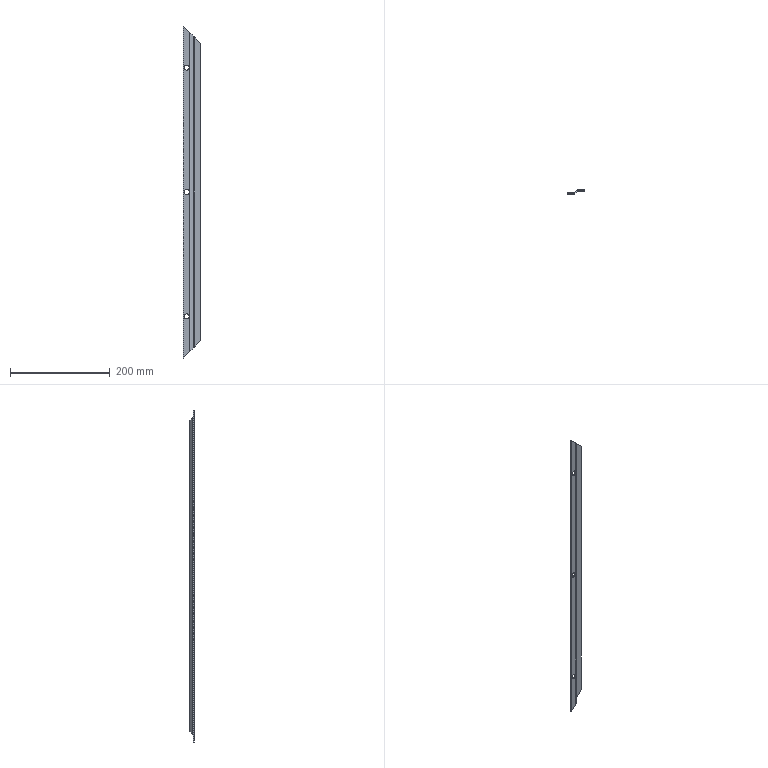Part | NX | features solid 2 | 1 solid | 28 faces | box 35 x 8.5 x 667 mm | volume 46692 mm3 | plane 14 | cylinder 10 | spline 4 | commonest cylinder face diameters 10 x6 4 x2 8 x2
STEP:
#1=CARTESIAN_POINT('',(-158.,-1615.,669.816));
#2=VERTEX_POINT('',#1);
#3=CARTESIAN_POINT('',(-158.,-1613.,669.816));
#4=VERTEX_POINT('',#3);
#5=CARTESIAN_POINT('',(-158.,-2280.972,669.816));
#6=DIRECTION('',(0.,1.,0.));
#7=VECTOR('',#6,1000.);
#8=LINE('',#5,#7);
#9=EDGE_CURVE('',#2,#4,#8,.T.);
#10=ORIENTED_EDGE('',*,*,#9,.F.);
#11=CARTESIAN_POINT('',(-168.,-1615.,669.816));
#12=VERTEX_POINT('',#11);
#13=CARTESIAN_POINT('',(-163.,-1615.,669.816));
#14=DIRECTION('',(0.,-1.,0.));
#15=DIRECTION('',(1.,0.,0.));
#16=AXIS2_PLACEMENT_3D('',#13,#14,#15);
#17=CIRCLE('',#16,5.);
#18=EDGE_CURVE('',#2,#12,#17,.T.);
#19=ORIENTED_EDGE('',*,*,#18,.T.);
#20=CARTESIAN_POINT('',(-168.,-1613.,669.816));
#21=VERTEX_POINT('',#20);
#22=CARTESIAN_POINT('',(-168.,-2280.972,669.816));
#23=DIRECTION('',(0.,1.,0.));
#24=VECTOR('',#23,1000.);
#25=LINE('',#22,#24);
#26=EDGE_CURVE('',#21,#12,#25,.F.);
#27=ORIENTED_EDGE('',*,*,#26,.F.);
#28=CARTESIAN_POINT('',(-163.,-1613.,669.816));
#29=DIRECTION('',(0.,1.,0.));
#30=DIRECTION('',(0.,0.,1.));
#31=AXIS2_PLACEMENT_3D('',#28,#29,#30);
#32=CIRCLE('',#31,5.);
#33=EDGE_CURVE('',#21,#4,#32,.T.);
#34=ORIENTED_EDGE('',*,*,#33,.T.);
#35=EDGE_LOOP('',(#10,#19,#27,#34));
#36=FACE_BOUND('',#35,.T.);
#37=CARTESIAN_POINT('',(-163.,-2280.972,669.816));
#38=DIRECTION('',(0.,1.,0.));
#39=DIRECTION('',(-1.,0.,0.));
#40=AXIS2_PLACEMENT_3D('',#37,#38,#39);
#41=CYLINDRICAL_SURFACE('',#40,5.);
#42=ADVANCED_FACE('',(#36),#41,.F.);
#43=CARTESIAN_POINT('',(-158.,-1613.,919.816));
#44=VERTEX_POINT('',#43);
#45=CARTESIAN_POINT('',(-158.,-1615.,919.816));
#46=VERTEX_POINT('',#45);
#47=CARTESIAN_POINT('',(-158.,-2280.972,919.816));
#48=DIRECTION('',(0.,1.,0.));
#49=VECTOR('',#48,1000.);
#50=LINE('',#47,#49);
#51=EDGE_CURVE('',#44,#46,#50,.F.);
#52=ORIENTED_EDGE('',*,*,#51,.T.);
#53=CARTESIAN_POINT('',(-168.,-1615.,919.816));
#54=VERTEX_POINT('',#53);
#55=CARTESIAN_POINT('',(-163.,-1615.,919.816));
#56=DIRECTION('',(0.,-1.,0.));
#57=DIRECTION('',(1.,0.,0.));
#58=AXIS2_PLACEMENT_3D('',#55,#56,#57);
#59=CIRCLE('',#58,5.);
#60=EDGE_CURVE('',#46,#54,#59,.T.);
#61=ORIENTED_EDGE('',*,*,#60,.T.);
#62=CARTESIAN_POINT('',(-168.,-1613.,919.816));
#63=VERTEX_POINT('',#62);
#64=CARTESIAN_POINT('',(-168.,-2280.972,919.816));
#65=DIRECTION('',(0.,1.,0.));
#66=VECTOR('',#65,1000.);
#67=LINE('',#64,#66);
#68=EDGE_CURVE('',#54,#63,#67,.T.);
#69=ORIENTED_EDGE('',*,*,#68,.T.);
#70=CARTESIAN_POINT('',(-163.,-1613.,919.816));
#71=DIRECTION('',(0.,1.,0.));
#72=DIRECTION('',(0.,0.,1.));
#73=AXIS2_PLACEMENT_3D('',#70,#71,#72);
#74=CIRCLE('',#73,5.);
#75=EDGE_CURVE('',#63,#44,#74,.T.);
#76=ORIENTED_EDGE('',*,*,#75,.T.);
#77=EDGE_LOOP('',(#52,#61,#69,#76));
#78=FACE_BOUND('',#77,.T.);
#79=CARTESIAN_POINT('',(-163.,-2280.972,919.816));
#80=DIRECTION('',(0.,1.,0.));
#81=DIRECTION('',(-1.,0.,0.));
#82=AXIS2_PLACEMENT_3D('',#79,#80,#81);
#83=CYLINDRICAL_SURFACE('',#82,5.);
#84=ADVANCED_FACE('',(#78),#83,.F.);
#85=CARTESIAN_POINT('',(-158.,-1613.,419.816));
#86=VERTEX_POINT('',#85);
#87=CARTESIAN_POINT('',(-158.,-1615.,419.816));
#88=VERTEX_POINT('',#87);
#89=CARTESIAN_POINT('',(-158.,-2280.972,419.816));
#90=DIRECTION('',(0.,1.,0.));
#91=VECTOR('',#90,1000.);
#92=LINE('',#89,#91);
#93=EDGE_CURVE('',#86,#88,#92,.F.);
#94=ORIENTED_EDGE('',*,*,#93,.T.);
#95=CARTESIAN_POINT('',(-168.,-1615.,419.816));
#96=VERTEX_POINT('',#95);
#97=CARTESIAN_POINT('',(-163.,-1615.,419.816));
#98=DIRECTION('',(0.,-1.,0.));
#99=DIRECTION('',(1.,0.,0.));
#100=AXIS2_PLACEMENT_3D('',#97,#98,#99);
#101=CIRCLE('',#100,5.);
#102=EDGE_CURVE('',#88,#96,#101,.T.);
#103=ORIENTED_EDGE('',*,*,#102,.T.);
#104=CARTESIAN_POINT('',(-168.,-1613.,419.816));
#105=VERTEX_POINT('',#104);
#106=CARTESIAN_POINT('',(-168.,-2280.972,419.816));
#107=DIRECTION('',(0.,1.,0.));
#108=VECTOR('',#107,1000.);
#109=LINE('',#106,#108);
#110=EDGE_CURVE('',#96,#105,#109,.T.);
#111=ORIENTED_EDGE('',*,*,#110,.T.);
#112=CARTESIAN_POINT('',(-163.,-1613.,419.816));
#113=DIRECTION('',(0.,1.,0.));
#114=DIRECTION('',(0.,0.,1.));
#115=AXIS2_PLACEMENT_3D('',#112,#113,#114);
#116=CIRCLE('',#115,5.);
#117=EDGE_CURVE('',#105,#86,#116,.T.);
#118=ORIENTED_EDGE('',*,*,#117,.T.);
#119=EDGE_LOOP('',(#94,#103,#111,#118));
#120=FACE_BOUND('',#119,.T.);
#121=CARTESIAN_POINT('',(-163.,-2280.972,419.816));
#122=DIRECTION('',(0.,1.,0.));
#123=DIRECTION('',(-1.,0.,0.));
#124=AXIS2_PLACEMENT_3D('',#121,#122,#123);
#125=CYLINDRICAL_SURFACE('',#124,5.);
#126=ADVANCED_FACE('',(#120),#125,.F.);
#127=CARTESIAN_POINT('',(-157.571,-1613.,348.745));
#128=VERTEX_POINT('',#127);
#129=CARTESIAN_POINT('',(-157.571,-1615.,348.745));
#130=VERTEX_POINT('',#129);
#131=CARTESIAN_POINT('',(-157.571,-1615.,348.745));
#132=DIRECTION('',(0.,-1.,0.));
#133=VECTOR('',#132,1000.);
#134=LINE('',#131,#133);
#135=EDGE_CURVE('',#128,#130,#134,.T.);
#136=ORIENTED_EDGE('',*,*,#135,.T.);
#137=CARTESIAN_POINT('',(-170.,-1615.,336.316));
#138=VERTEX_POINT('',#137);
#139=CARTESIAN_POINT('',(1171.,-1615.,1677.316));
#140=DIRECTION('',(-0.7071,0.,-0.7071));
#141=VECTOR('',#140,1000.);
#142=LINE('',#139,#141);
#143=EDGE_CURVE('',#130,#138,#142,.T.);
#144=ORIENTED_EDGE('',*,*,#143,.T.);
#145=CARTESIAN_POINT('',(-170.,-1613.,336.316));
#146=VERTEX_POINT('',#145);
#147=CARTESIAN_POINT('',(-170.,-1615.,336.316));
#148=DIRECTION('',(0.,-1.,0.));
#149=VECTOR('',#148,1000.);
#150=LINE('',#147,#149);
#151=EDGE_CURVE('',#146,#138,#150,.T.);
#152=ORIENTED_EDGE('',*,*,#151,.F.);
#153=CARTESIAN_POINT('',(1171.,-1613.,1677.316));
#154=DIRECTION('',(-0.7071,0.,-0.7071));
#155=VECTOR('',#154,1000.);
#156=LINE('',#153,#155);
#157=EDGE_CURVE('',#128,#146,#156,.T.);
#158=ORIENTED_EDGE('',*,*,#157,.F.);
#159=EDGE_LOOP('',(#136,#144,#152,#158));
#160=FACE_BOUND('',#159,.T.);
#161=CARTESIAN_POINT('',(1171.,-1615.,1677.316));
#162=DIRECTION('',(-0.7071,0.,0.7071));
#163=DIRECTION('',(0.,1.,0.));
#164=AXIS2_PLACEMENT_3D('',#161,#162,#163);
#165=PLANE('',#164);
#166=ADVANCED_FACE('',(#160),#165,.F.);
#167=CARTESIAN_POINT('',(-156.21,-1612.466,351.467));
#168=VERTEX_POINT('',#167);
#169=CARTESIAN_POINT('',(-154.849,-1613.931,351.467));
#170=VERTEX_POINT('',#169);
#171=CARTESIAN_POINT('',(-154.849,-1613.931,351.467));
#172=DIRECTION('',(0.6805,-0.7328,0.));
#173=VECTOR('',#172,1000.);
#174=LINE('',#171,#173);
#175=EDGE_CURVE('',#168,#170,#174,.T.);
#176=ORIENTED_EDGE('',*,*,#175,.T.);
#177=CARTESIAN_POINT('',(-154.849,-1613.931,351.467));
#178=CARTESIAN_POINT('',(-155.598,-1614.626,350.718));
#179=CARTESIAN_POINT('',(-156.549,-1615.,349.767));
#180=CARTESIAN_POINT('',(-157.571,-1615.,348.745));
#181=(BOUNDED_CURVE()B_SPLINE_CURVE(3,(#177,#178,#179,#180),.UNSPECIFIED.,.F.,.F.)B_SPLINE_CURVE_WITH_KNOTS((4,4),(3.964,4.712),.PIECEWISE_BEZIER_KNOTS.)CURVE()GEOMETRIC_REPRESENTATION_ITEM()RATIONAL_B_SPLINE_CURVE((1.,0.9539,0.9539,1.))REPRESENTATION_ITEM(''));
#182=EDGE_CURVE('',#170,#130,#181,.T.);
#183=ORIENTED_EDGE('',*,*,#182,.T.);
#184=ORIENTED_EDGE('',*,*,#135,.F.);
#185=CARTESIAN_POINT('',(-156.21,-1612.466,351.467));
#186=CARTESIAN_POINT('',(-156.584,-1612.813,350.718));
#187=CARTESIAN_POINT('',(-157.06,-1613.,349.767));
#188=CARTESIAN_POINT('',(-157.571,-1613.,348.745));
#189=(BOUNDED_CURVE()B_SPLINE_CURVE(3,(#185,#186,#187,#188),.UNSPECIFIED.,.F.,.F.)B_SPLINE_CURVE_WITH_KNOTS((4,4),(3.964,4.712),.PIECEWISE_BEZIER_KNOTS.)CURVE()GEOMETRIC_REPRESENTATION_ITEM()RATIONAL_B_SPLINE_CURVE((1.,0.9539,0.9539,1.))REPRESENTATION_ITEM(''));
#190=EDGE_CURVE('',#168,#128,#189,.T.);
#191=ORIENTED_EDGE('',*,*,#190,.F.);
#192=EDGE_LOOP('',(#176,#183,#184,#191));
#193=FACE_BOUND('',#192,.T.);
#194=CARTESIAN_POINT('',(-154.849,-1613.931,351.467));
#195=CARTESIAN_POINT('',(-155.303,-1613.443,351.467));
#196=CARTESIAN_POINT('',(-155.756,-1612.954,351.467));
#197=CARTESIAN_POINT('',(-156.21,-1612.466,351.467));
#198=CARTESIAN_POINT('',(-155.579,-1614.609,350.737));
#199=CARTESIAN_POINT('',(-155.911,-1614.007,350.737));
#200=CARTESIAN_POINT('',(-156.243,-1613.406,350.737));
#201=CARTESIAN_POINT('',(-156.575,-1612.804,350.737));
#202=CARTESIAN_POINT('',(-156.524,-1615.,349.793));
#203=CARTESIAN_POINT('',(-156.698,-1614.333,349.793));
#204=CARTESIAN_POINT('',(-156.873,-1613.667,349.793));
#205=CARTESIAN_POINT('',(-157.047,-1613.,349.793));
#206=CARTESIAN_POINT('',(-157.571,-1615.,348.745));
#207=CARTESIAN_POINT('',(-157.571,-1614.333,348.745));
#208=CARTESIAN_POINT('',(-157.571,-1613.667,348.745));
#209=CARTESIAN_POINT('',(-157.571,-1613.,348.745));
#210=(BOUNDED_SURFACE()B_SPLINE_SURFACE(3,3,((#194,#195,#196,#197),(#198,#199,#200,#201),(#202,#203,#204,#205),(#206,#207,#208,#209)),.RULED_SURF.,.F.,.F.,.F.)B_SPLINE_SURFACE_WITH_KNOTS((4,4),(4,4),(0.6518,0.75),(0.,1.),.PIECEWISE_BEZIER_KNOTS.)GEOMETRIC_REPRESENTATION_ITEM()RATIONAL_B_SPLINE_SURFACE(((0.5771,0.5771,0.5771,0.5771),(0.5257,0.5257,0.5257,0.5257),(0.5,0.5,0.5,0.5),(0.5,0.5,0.5,0.5)))REPRESENTATION_ITEM('')SURFACE());
#211=ADVANCED_FACE('',(#193),#210,.T.);
#212=CARTESIAN_POINT('',(-150.936,-1607.569,356.741));
#213=VERTEX_POINT('',#212);
#214=CARTESIAN_POINT('',(-149.576,-1609.034,356.741));
#215=VERTEX_POINT('',#214);
#216=CARTESIAN_POINT('',(-149.576,-1609.034,356.741));
#217=DIRECTION('',(0.6805,-0.7328,0.));
#218=VECTOR('',#217,1000.);
#219=LINE('',#216,#218);
#220=EDGE_CURVE('',#213,#215,#219,.T.);
#221=ORIENTED_EDGE('',*,*,#220,.T.);
#222=CARTESIAN_POINT('',(775.799,-749.758,1282.115));
#223=DIRECTION('',(-0.5911,-0.5489,-0.5911));
#224=VECTOR('',#223,1000.);
#225=LINE('',#222,#224);
#226=EDGE_CURVE('',#215,#170,#225,.T.);
#227=ORIENTED_EDGE('',*,*,#226,.T.);
#228=ORIENTED_EDGE('',*,*,#175,.F.);
#229=CARTESIAN_POINT('',(774.438,-748.293,1282.115));
#230=DIRECTION('',(-0.5911,-0.5489,-0.5911));
#231=VECTOR('',#230,1000.);
#232=LINE('',#229,#231);
#233=EDGE_CURVE('',#213,#168,#232,.T.);
#234=ORIENTED_EDGE('',*,*,#233,.F.);
#235=EDGE_LOOP('',(#221,#227,#228,#234));
#236=FACE_BOUND('',#235,.T.);
#237=CARTESIAN_POINT('',(775.799,-749.758,1282.115));
#238=DIRECTION('',(-0.4331,-0.4022,0.8066));
#239=DIRECTION('',(-0.6805,0.7328,0.));
#240=AXIS2_PLACEMENT_3D('',#237,#238,#239);
#241=PLANE('',#240);
#242=ADVANCED_FACE('',(#236),#241,.F.);
#243=CARTESIAN_POINT('',(-148.215,-1606.5,358.102));
#244=VERTEX_POINT('',#243);
#245=CARTESIAN_POINT('',(-148.215,-1608.5,358.102));
#246=VERTEX_POINT('',#245);
#247=CARTESIAN_POINT('',(-148.215,-1608.5,358.102));
#248=DIRECTION('',(0.,-1.,0.));
#249=VECTOR('',#248,1000.);
#250=LINE('',#247,#249);
#251=EDGE_CURVE('',#244,#246,#250,.T.);
#252=ORIENTED_EDGE('',*,*,#251,.T.);
#253=CARTESIAN_POINT('',(-148.215,-1608.5,358.102));
#254=CARTESIAN_POINT('',(-148.726,-1608.5,357.591));
#255=CARTESIAN_POINT('',(-149.201,-1608.687,357.115));
#256=CARTESIAN_POINT('',(-149.576,-1609.034,356.741));
#257=(BOUNDED_CURVE()B_SPLINE_CURVE(3,(#253,#254,#255,#256),.UNSPECIFIED.,.F.,.F.)B_SPLINE_CURVE_WITH_KNOTS((4,4),(4.712,5.461),.PIECEWISE_BEZIER_KNOTS.)CURVE()GEOMETRIC_REPRESENTATION_ITEM()RATIONAL_B_SPLINE_CURVE((1.,0.9539,0.9539,1.))REPRESENTATION_ITEM(''));
#258=EDGE_CURVE('',#246,#215,#257,.T.);
#259=ORIENTED_EDGE('',*,*,#258,.T.);
#260=ORIENTED_EDGE('',*,*,#220,.F.);
#261=CARTESIAN_POINT('',(-148.215,-1606.5,358.102));
#262=CARTESIAN_POINT('',(-149.236,-1606.5,357.591));
#263=CARTESIAN_POINT('',(-150.188,-1606.874,357.115));
#264=CARTESIAN_POINT('',(-150.936,-1607.569,356.741));
#265=(BOUNDED_CURVE()B_SPLINE_CURVE(3,(#261,#262,#263,#264),.UNSPECIFIED.,.F.,.F.)B_SPLINE_CURVE_WITH_KNOTS((4,4),(4.712,5.461),.PIECEWISE_BEZIER_KNOTS.)CURVE()GEOMETRIC_REPRESENTATION_ITEM()RATIONAL_B_SPLINE_CURVE((1.,0.9539,0.9539,1.))REPRESENTATION_ITEM(''));
#266=EDGE_CURVE('',#244,#213,#265,.T.);
#267=ORIENTED_EDGE('',*,*,#266,.F.);
#268=EDGE_LOOP('',(#252,#259,#260,#267));
#269=FACE_BOUND('',#268,.T.);
#270=CARTESIAN_POINT('',(-148.215,-1608.5,358.102));
#271=CARTESIAN_POINT('',(-148.215,-1607.833,358.102));
#272=CARTESIAN_POINT('',(-148.215,-1607.167,358.102));
#273=CARTESIAN_POINT('',(-148.215,-1606.5,358.102));
#274=CARTESIAN_POINT('',(-148.738,-1608.5,357.578));
#275=CARTESIAN_POINT('',(-148.913,-1607.833,357.578));
#276=CARTESIAN_POINT('',(-149.087,-1607.167,357.578));
#277=CARTESIAN_POINT('',(-149.262,-1606.5,357.578));
#278=CARTESIAN_POINT('',(-149.211,-1608.696,357.106));
#279=CARTESIAN_POINT('',(-149.543,-1608.094,357.106));
#280=CARTESIAN_POINT('',(-149.875,-1607.493,357.106));
#281=CARTESIAN_POINT('',(-150.207,-1606.891,357.106));
#282=CARTESIAN_POINT('',(-149.576,-1609.034,356.741));
#283=CARTESIAN_POINT('',(-150.029,-1608.546,356.741));
#284=CARTESIAN_POINT('',(-150.483,-1608.057,356.741));
#285=CARTESIAN_POINT('',(-150.936,-1607.569,356.741));
#286=(BOUNDED_SURFACE()B_SPLINE_SURFACE(3,3,((#270,#271,#272,#273),(#274,#275,#276,#277),(#278,#279,#280,#281),(#282,#283,#284,#285)),.UNSPECIFIED.,.F.,.F.,.F.)B_SPLINE_SURFACE_WITH_KNOTS((4,4),(4,4),(0.75,0.8482),(0.,1.),.PIECEWISE_BEZIER_KNOTS.)GEOMETRIC_REPRESENTATION_ITEM()RATIONAL_B_SPLINE_SURFACE(((0.5,0.5,0.5,0.5),(0.5,0.5,0.5,0.5),(0.5257,0.5257,0.5257,0.5257),(0.5771,0.5771,0.5771,0.5771)))REPRESENTATION_ITEM('')SURFACE());
#287=ADVANCED_FACE('',(#269),#286,.T.);
#288=CARTESIAN_POINT('',(-135.,-1606.5,371.316));
#289=VERTEX_POINT('',#288);
#290=CARTESIAN_POINT('',(-135.,-1608.5,371.316));
#291=VERTEX_POINT('',#290);
#292=CARTESIAN_POINT('',(-135.,-1608.5,371.316));
#293=DIRECTION('',(0.,-1.,0.));
#294=VECTOR('',#293,1000.);
#295=LINE('',#292,#294);
#296=EDGE_CURVE('',#289,#291,#295,.T.);
#297=ORIENTED_EDGE('',*,*,#296,.T.);
#298=CARTESIAN_POINT('',(1181.5,-1608.5,1687.816));
#299=DIRECTION('',(-0.7071,0.,-0.7071));
#300=VECTOR('',#299,1000.);
#301=LINE('',#298,#300);
#302=EDGE_CURVE('',#291,#246,#301,.T.);
#303=ORIENTED_EDGE('',*,*,#302,.T.);
#304=ORIENTED_EDGE('',*,*,#251,.F.);
#305=CARTESIAN_POINT('',(1181.5,-1606.5,1687.816));
#306=DIRECTION('',(-0.7071,0.,-0.7071));
#307=VECTOR('',#306,1000.);
#308=LINE('',#305,#307);
#309=EDGE_CURVE('',#289,#244,#308,.T.);
#310=ORIENTED_EDGE('',*,*,#309,.F.);
#311=EDGE_LOOP('',(#297,#303,#304,#310));
#312=FACE_BOUND('',#311,.T.);
#313=CARTESIAN_POINT('',(1181.5,-1608.5,1687.816));
#314=DIRECTION('',(-0.7071,0.,0.7071));
#315=DIRECTION('',(0.,1.,0.));
#316=AXIS2_PLACEMENT_3D('',#313,#314,#315);
#317=PLANE('',#316);
#318=ADVANCED_FACE('',(#312),#317,.F.);
#319=CARTESIAN_POINT('',(-170.,-1613.,1003.316));
#320=VERTEX_POINT('',#319);
#321=CARTESIAN_POINT('',(-157.571,-1613.,990.887));
#322=VERTEX_POINT('',#321);
#323=CARTESIAN_POINT('',(-1163.5,-1613.,1996.816));
#324=DIRECTION('',(0.7071,0.,-0.7071));
#325=VECTOR('',#324,1000.);
#326=LINE('',#323,#325);
#327=EDGE_CURVE('',#320,#322,#326,.T.);
#328=ORIENTED_EDGE('',*,*,#327,.F.);
#329=CARTESIAN_POINT('',(-170.,-1615.,1003.316));
#330=VERTEX_POINT('',#329);
#331=CARTESIAN_POINT('',(-170.,-1615.,1003.316));
#332=DIRECTION('',(0.,-1.,0.));
#333=VECTOR('',#332,1000.);
#334=LINE('',#331,#333);
#335=EDGE_CURVE('',#320,#330,#334,.T.);
#336=ORIENTED_EDGE('',*,*,#335,.T.);
#337=CARTESIAN_POINT('',(-157.571,-1615.,990.887));
#338=VERTEX_POINT('',#337);
#339=CARTESIAN_POINT('',(-1163.5,-1615.,1996.816));
#340=DIRECTION('',(0.7071,0.,-0.7071));
#341=VECTOR('',#340,1000.);
#342=LINE('',#339,#341);
#343=EDGE_CURVE('',#330,#338,#342,.T.);
#344=ORIENTED_EDGE('',*,*,#343,.T.);
#345=CARTESIAN_POINT('',(-157.571,-1615.,990.887));
#346=DIRECTION('',(0.,-1.,0.));
#347=VECTOR('',#346,1000.);
#348=LINE('',#345,#347);
#349=EDGE_CURVE('',#322,#338,#348,.T.);
#350=ORIENTED_EDGE('',*,*,#349,.F.);
#351=EDGE_LOOP('',(#328,#336,#344,#350));
#352=FACE_BOUND('',#351,.T.);
#353=CARTESIAN_POINT('',(-1163.5,-1615.,1996.816));
#354=DIRECTION('',(-0.7071,0.,-0.7071));
#355=DIRECTION('',(-0.7071,0.,0.7071));
#356=AXIS2_PLACEMENT_3D('',#353,#354,#355);
#357=PLANE('',#356);
#358=ADVANCED_FACE('',(#352),#357,.F.);
#359=CARTESIAN_POINT('',(-148.215,-1606.5,981.531));
#360=VERTEX_POINT('',#359);
#361=CARTESIAN_POINT('',(-148.215,-1608.5,981.531));
#362=VERTEX_POINT('',#361);
#363=CARTESIAN_POINT('',(-148.215,-1608.5,981.531));
#364=DIRECTION('',(0.,-1.,0.));
#365=VECTOR('',#364,1000.);
#366=LINE('',#363,#365);
#367=EDGE_CURVE('',#360,#362,#366,.T.);
#368=ORIENTED_EDGE('',*,*,#367,.T.);
#369=CARTESIAN_POINT('',(-135.,-1608.5,968.316));
#370=VERTEX_POINT('',#369);
#371=CARTESIAN_POINT('',(-1153.,-1608.5,1986.316));
#372=DIRECTION('',(0.7071,0.,-0.7071));
#373=VECTOR('',#372,1000.);
#374=LINE('',#371,#373);
#375=EDGE_CURVE('',#362,#370,#374,.T.);
#376=ORIENTED_EDGE('',*,*,#375,.T.);
#377=CARTESIAN_POINT('',(-135.,-1606.5,968.316));
#378=VERTEX_POINT('',#377);
#379=CARTESIAN_POINT('',(-135.,-1608.5,968.316));
#380=DIRECTION('',(0.,-1.,0.));
#381=VECTOR('',#380,1000.);
#382=LINE('',#379,#381);
#383=EDGE_CURVE('',#378,#370,#382,.T.);
#384=ORIENTED_EDGE('',*,*,#383,.F.);
#385=CARTESIAN_POINT('',(-1153.,-1606.5,1986.316));
#386=DIRECTION('',(0.7071,0.,-0.7071));
#387=VECTOR('',#386,1000.);
#388=LINE('',#385,#387);
#389=EDGE_CURVE('',#360,#378,#388,.T.);
#390=ORIENTED_EDGE('',*,*,#389,.F.);
#391=EDGE_LOOP('',(#368,#376,#384,#390));
#392=FACE_BOUND('',#391,.T.);
#393=CARTESIAN_POINT('',(-1153.,-1608.5,1986.316));
#394=DIRECTION('',(-0.7071,0.,-0.7071));
#395=DIRECTION('',(-0.7071,0.,0.7071));
#396=AXIS2_PLACEMENT_3D('',#393,#394,#395);
#397=PLANE('',#396);
#398=ADVANCED_FACE('',(#392),#397,.F.);
#399=CARTESIAN_POINT('',(-150.936,-1607.569,982.892));
#400=VERTEX_POINT('',#399);
#401=CARTESIAN_POINT('',(-149.576,-1609.034,982.892));
#402=VERTEX_POINT('',#401);
#403=CARTESIAN_POINT('',(-149.576,-1609.034,982.892));
#404=DIRECTION('',(0.6805,-0.7328,0.));
#405=VECTOR('',#404,1000.);
#406=LINE('',#403,#405);
#407=EDGE_CURVE('',#400,#402,#406,.T.);
#408=ORIENTED_EDGE('',*,*,#407,.T.);
#409=CARTESIAN_POINT('',(-149.576,-1609.034,982.892));
#410=CARTESIAN_POINT('',(-149.201,-1608.687,982.517));
#411=CARTESIAN_POINT('',(-148.726,-1608.5,982.042));
#412=CARTESIAN_POINT('',(-148.215,-1608.5,981.531));
#413=(BOUNDED_CURVE()B_SPLINE_CURVE(3,(#409,#410,#411,#412),.UNSPECIFIED.,.F.,.F.)B_SPLINE_CURVE_WITH_KNOTS((4,4),(3.964,4.712),.PIECEWISE_BEZIER_KNOTS.)CURVE()GEOMETRIC_REPRESENTATION_ITEM()RATIONAL_B_SPLINE_CURVE((1.,0.9539,0.9539,1.))REPRESENTATION_ITEM(''));
#414=EDGE_CURVE('',#402,#362,#413,.T.);
#415=ORIENTED_EDGE('',*,*,#414,.T.);
#416=ORIENTED_EDGE('',*,*,#367,.F.);
#417=CARTESIAN_POINT('',(-150.936,-1607.569,982.892));
#418=CARTESIAN_POINT('',(-150.188,-1606.874,982.517));
#419=CARTESIAN_POINT('',(-149.236,-1606.5,982.042));
#420=CARTESIAN_POINT('',(-148.215,-1606.5,981.531));
#421=(BOUNDED_CURVE()B_SPLINE_CURVE(3,(#417,#418,#419,#420),.UNSPECIFIED.,.F.,.F.)B_SPLINE_CURVE_WITH_KNOTS((4,4),(3.964,4.712),.PIECEWISE_BEZIER_KNOTS.)CURVE()GEOMETRIC_REPRESENTATION_ITEM()RATIONAL_B_SPLINE_CURVE((1.,0.9539,0.9539,1.))REPRESENTATION_ITEM(''));
#422=EDGE_CURVE('',#400,#360,#421,.T.);
#423=ORIENTED_EDGE('',*,*,#422,.F.);
#424=EDGE_LOOP('',(#408,#415,#416,#423));
#425=FACE_BOUND('',#424,.T.);
#426=CARTESIAN_POINT('',(-149.576,-1609.034,982.892));
#427=CARTESIAN_POINT('',(-150.029,-1608.546,982.892));
#428=CARTESIAN_POINT('',(-150.483,-1608.057,982.892));
#429=CARTESIAN_POINT('',(-150.936,-1607.569,982.892));
#430=CARTESIAN_POINT('',(-149.211,-1608.696,982.527));
#431=CARTESIAN_POINT('',(-149.543,-1608.094,982.527));
#432=CARTESIAN_POINT('',(-149.875,-1607.493,982.527));
#433=CARTESIAN_POINT('',(-150.207,-1606.891,982.527));
#434=CARTESIAN_POINT('',(-148.738,-1608.5,982.054));
#435=CARTESIAN_POINT('',(-148.913,-1607.833,982.054));
#436=CARTESIAN_POINT('',(-149.087,-1607.167,982.054));
#437=CARTESIAN_POINT('',(-149.262,-1606.5,982.054));
#438=CARTESIAN_POINT('',(-148.215,-1608.5,981.531));
#439=CARTESIAN_POINT('',(-148.215,-1607.833,981.531));
#440=CARTESIAN_POINT('',(-148.215,-1607.167,981.531));
#441=CARTESIAN_POINT('',(-148.215,-1606.5,981.531));
#442=(BOUNDED_SURFACE()B_SPLINE_SURFACE(3,3,((#426,#427,#428,#429),(#430,#431,#432,#433),(#434,#435,#436,#437),(#438,#439,#440,#441)),.UNSPECIFIED.,.F.,.F.,.F.)B_SPLINE_SURFACE_WITH_KNOTS((4,4),(4,4),(0.6518,0.75),(0.,1.),.PIECEWISE_BEZIER_KNOTS.)GEOMETRIC_REPRESENTATION_ITEM()RATIONAL_B_SPLINE_SURFACE(((0.5771,0.5771,0.5771,0.5771),(0.5257,0.5257,0.5257,0.5257),(0.5,0.5,0.5,0.5),(0.5,0.5,0.5,0.5)))REPRESENTATION_ITEM('')SURFACE());
#443=ADVANCED_FACE('',(#425),#442,.T.);
#444=CARTESIAN_POINT('',(-156.21,-1612.466,988.165));
#445=VERTEX_POINT('',#444);
#446=CARTESIAN_POINT('',(-154.849,-1613.931,988.165));
#447=VERTEX_POINT('',#446);
#448=CARTESIAN_POINT('',(-154.849,-1613.931,988.165));
#449=DIRECTION('',(0.6805,-0.7328,0.));
#450=VECTOR('',#449,1000.);
#451=LINE('',#448,#450);
#452=EDGE_CURVE('',#445,#447,#451,.T.);
#453=ORIENTED_EDGE('',*,*,#452,.T.);
#454=CARTESIAN_POINT('',(-855.439,-2264.479,1688.755));
#455=DIRECTION('',(0.5911,0.5489,-0.5911));
#456=VECTOR('',#455,1000.);
#457=LINE('',#454,#456);
#458=EDGE_CURVE('',#447,#402,#457,.T.);
#459=ORIENTED_EDGE('',*,*,#458,.T.);
#460=ORIENTED_EDGE('',*,*,#407,.F.);
#461=CARTESIAN_POINT('',(-856.799,-2263.013,1688.755));
#462=DIRECTION('',(0.5911,0.5489,-0.5911));
#463=VECTOR('',#462,1000.);
#464=LINE('',#461,#463);
#465=EDGE_CURVE('',#445,#400,#464,.T.);
#466=ORIENTED_EDGE('',*,*,#465,.F.);
#467=EDGE_LOOP('',(#453,#459,#460,#466));
#468=FACE_BOUND('',#467,.T.);
#469=CARTESIAN_POINT('',(-855.439,-2264.479,1688.755));
#470=DIRECTION('',(-0.4331,-0.4022,-0.8066));
#471=DIRECTION('',(-0.881,0.,0.4731));
#472=AXIS2_PLACEMENT_3D('',#469,#470,#471);
#473=PLANE('',#472);
#474=ADVANCED_FACE('',(#468),#473,.F.);
#475=ORIENTED_EDGE('',*,*,#349,.T.);
#476=CARTESIAN_POINT('',(-157.571,-1615.,990.887));
#477=CARTESIAN_POINT('',(-156.549,-1615.,989.865));
#478=CARTESIAN_POINT('',(-155.598,-1614.626,988.914));
#479=CARTESIAN_POINT('',(-154.849,-1613.931,988.165));
#480=(BOUNDED_CURVE()B_SPLINE_CURVE(3,(#476,#477,#478,#479),.UNSPECIFIED.,.F.,.F.)B_SPLINE_CURVE_WITH_KNOTS((4,4),(4.712,5.461),.PIECEWISE_BEZIER_KNOTS.)CURVE()GEOMETRIC_REPRESENTATION_ITEM()RATIONAL_B_SPLINE_CURVE((1.,0.9539,0.9539,1.))REPRESENTATION_ITEM(''));
#481=EDGE_CURVE('',#338,#447,#480,.T.);
#482=ORIENTED_EDGE('',*,*,#481,.T.);
#483=ORIENTED_EDGE('',*,*,#452,.F.);
#484=CARTESIAN_POINT('',(-157.571,-1613.,990.887));
#485=CARTESIAN_POINT('',(-157.06,-1613.,989.865));
#486=CARTESIAN_POINT('',(-156.584,-1612.813,988.914));
#487=CARTESIAN_POINT('',(-156.21,-1612.466,988.165));
#488=(BOUNDED_CURVE()B_SPLINE_CURVE(3,(#484,#485,#486,#487),.UNSPECIFIED.,.F.,.F.)B_SPLINE_CURVE_WITH_KNOTS((4,4),(4.712,5.461),.PIECEWISE_BEZIER_KNOTS.)CURVE()GEOMETRIC_REPRESENTATION_ITEM()RATIONAL_B_SPLINE_CURVE((1.,0.9539,0.9539,1.))REPRESENTATION_ITEM(''));
#489=EDGE_CURVE('',#322,#445,#488,.T.);
#490=ORIENTED_EDGE('',*,*,#489,.F.);
#491=EDGE_LOOP('',(#475,#482,#483,#490));
#492=FACE_BOUND('',#491,.T.);
#493=CARTESIAN_POINT('',(-157.571,-1615.,990.887));
#494=CARTESIAN_POINT('',(-157.571,-1614.333,990.887));
#495=CARTESIAN_POINT('',(-157.571,-1613.667,990.887));
#496=CARTESIAN_POINT('',(-157.571,-1613.,990.887));
#497=CARTESIAN_POINT('',(-156.524,-1615.,989.84));
#498=CARTESIAN_POINT('',(-156.698,-1614.333,989.84));
#499=CARTESIAN_POINT('',(-156.873,-1613.667,989.84));
#500=CARTESIAN_POINT('',(-157.047,-1613.,989.84));
#501=CARTESIAN_POINT('',(-155.579,-1614.609,988.895));
#502=CARTESIAN_POINT('',(-155.911,-1614.007,988.895));
#503=CARTESIAN_POINT('',(-156.243,-1613.406,988.895));
#504=CARTESIAN_POINT('',(-156.575,-1612.804,988.895));
#505=CARTESIAN_POINT('',(-154.849,-1613.931,988.165));
#506=CARTESIAN_POINT('',(-155.303,-1613.443,988.165));
#507=CARTESIAN_POINT('',(-155.756,-1612.954,988.165));
#508=CARTESIAN_POINT('',(-156.21,-1612.466,988.165));
#509=(BOUNDED_SURFACE()B_SPLINE_SURFACE(3,3,((#493,#494,#495,#496),(#497,#498,#499,#500),(#501,#502,#503,#504),(#505,#506,#507,#508)),.UNSPECIFIED.,.F.,.F.,.F.)B_SPLINE_SURFACE_WITH_KNOTS((4,4),(4,4),(0.75,0.8482),(0.,1.),.PIECEWISE_BEZIER_KNOTS.)GEOMETRIC_REPRESENTATION_ITEM()RATIONAL_B_SPLINE_SURFACE(((0.5,0.5,0.5,0.5),(0.5,0.5,0.5,0.5),(0.5257,0.5257,0.5257,0.5257),(0.5771,0.5771,0.5771,0.5771)))REPRESENTATION_ITEM('')SURFACE());
#510=ADVANCED_FACE('',(#492),#509,.T.);
#511=ORIENTED_EDGE('',*,*,#117,.F.);
#512=CARTESIAN_POINT('',(-163.,-1613.,419.816));
#513=DIRECTION('',(0.,1.,0.));
#514=DIRECTION('',(0.,0.,1.));
#515=AXIS2_PLACEMENT_3D('',#512,#513,#514);
#516=CIRCLE('',#515,5.);
#517=EDGE_CURVE('',#86,#105,#516,.T.);
#518=ORIENTED_EDGE('',*,*,#517,.F.);
#519=EDGE_LOOP('',(#511,#518));
#520=FACE_BOUND('',#519,.T.);
#521=ORIENTED_EDGE('',*,*,#75,.F.);
#522=CARTESIAN_POINT('',(-163.,-1613.,919.816));
#523=DIRECTION('',(0.,1.,0.));
#524=DIRECTION('',(0.,0.,1.));
#525=AXIS2_PLACEMENT_3D('',#522,#523,#524);
#526=CIRCLE('',#525,5.);
#527=EDGE_CURVE('',#44,#63,#526,.T.);
#528=ORIENTED_EDGE('',*,*,#527,.F.);
#529=EDGE_LOOP('',(#521,#528));
#530=FACE_BOUND('',#529,.T.);
#531=ORIENTED_EDGE('',*,*,#33,.F.);
#532=CARTESIAN_POINT('',(-163.,-1613.,669.816));
#533=DIRECTION('',(0.,1.,0.));
#534=DIRECTION('',(0.,0.,1.));
#535=AXIS2_PLACEMENT_3D('',#532,#533,#534);
#536=CIRCLE('',#535,5.);
#537=EDGE_CURVE('',#4,#21,#536,.T.);
#538=ORIENTED_EDGE('',*,*,#537,.F.);
#539=EDGE_LOOP('',(#531,#538));
#540=FACE_BOUND('',#539,.T.);
#541=CARTESIAN_POINT('',(-157.571,-1613.,3004.316));
#542=DIRECTION('',(0.,0.,-1.));
#543=VECTOR('',#542,1000.);
#544=LINE('',#541,#543);
#545=EDGE_CURVE('',#322,#128,#544,.T.);
#546=ORIENTED_EDGE('',*,*,#545,.T.);
#547=ORIENTED_EDGE('',*,*,#157,.T.);
#548=CARTESIAN_POINT('',(-170.,-1613.,3004.316));
#549=DIRECTION('',(0.,0.,-1.));
#550=VECTOR('',#549,1000.);
#551=LINE('',#548,#550);
#552=EDGE_CURVE('',#320,#146,#551,.T.);
#553=ORIENTED_EDGE('',*,*,#552,.F.);
#554=ORIENTED_EDGE('',*,*,#327,.T.);
#555=EDGE_LOOP('',(#546,#547,#553,#554));
#556=FACE_BOUND('',#555,.T.);
#557=CARTESIAN_POINT('',(-156.,-1613.,3004.316));
#558=DIRECTION('',(0.,-1.,0.));
#559=DIRECTION('',(0.,0.,-1.));
#560=AXIS2_PLACEMENT_3D('',#557,#558,#559);
#561=PLANE('',#560);
#562=ADVANCED_FACE('',(#520,#530,#540,#556),#561,.F.);
#563=CARTESIAN_POINT('',(-156.21,-1612.466,3004.316));
#564=DIRECTION('',(0.,0.,-1.));
#565=VECTOR('',#564,1000.);
#566=LINE('',#563,#565);
#567=EDGE_CURVE('',#445,#168,#566,.T.);
#568=ORIENTED_EDGE('',*,*,#567,.T.);
#569=ORIENTED_EDGE('',*,*,#190,.T.);
#570=ORIENTED_EDGE('',*,*,#545,.F.);
#571=ORIENTED_EDGE('',*,*,#489,.T.);
#572=EDGE_LOOP('',(#568,#569,#570,#571));
#573=FACE_BOUND('',#572,.T.);
#574=CARTESIAN_POINT('',(-157.571,-1611.,3004.316));
#575=DIRECTION('',(0.,0.,-1.));
#576=DIRECTION('',(0.,-1.,0.));
#577=AXIS2_PLACEMENT_3D('',#574,#575,#576);
#578=CYLINDRICAL_SURFACE('',#577,2.);
#579=ADVANCED_FACE('',(#573),#578,.F.);
#580=CARTESIAN_POINT('',(-150.936,-1607.569,3004.316));
#581=DIRECTION('',(0.,0.,-1.));
#582=VECTOR('',#581,1000.);
#583=LINE('',#580,#582);
#584=EDGE_CURVE('',#400,#213,#583,.T.);
#585=ORIENTED_EDGE('',*,*,#584,.T.);
#586=ORIENTED_EDGE('',*,*,#233,.T.);
#587=ORIENTED_EDGE('',*,*,#567,.F.);
#588=ORIENTED_EDGE('',*,*,#465,.T.);
#589=EDGE_LOOP('',(#585,#586,#587,#588));
#590=FACE_BOUND('',#589,.T.);
#591=CARTESIAN_POINT('',(-150.361,-1607.034,3004.316));
#592=DIRECTION('',(0.6805,-0.7328,0.));
#593=DIRECTION('',(0.,0.,-1.));
#594=AXIS2_PLACEMENT_3D('',#591,#592,#593);
#595=PLANE('',#594);
#596=ADVANCED_FACE('',(#590),#595,.F.);
#597=CARTESIAN_POINT('',(-148.215,-1606.5,3004.316));
#598=DIRECTION('',(0.,0.,-1.));
#599=VECTOR('',#598,1000.);
#600=LINE('',#597,#599);
#601=EDGE_CURVE('',#360,#244,#600,.T.);
#602=ORIENTED_EDGE('',*,*,#601,.T.);
#603=ORIENTED_EDGE('',*,*,#266,.T.);
#604=ORIENTED_EDGE('',*,*,#584,.F.);
#605=ORIENTED_EDGE('',*,*,#422,.T.);
#606=EDGE_LOOP('',(#602,#603,#604,#605));
#607=FACE_BOUND('',#606,.T.);
#608=CARTESIAN_POINT('',(-148.215,-1610.5,3004.316));
#609=DIRECTION('',(0.,0.,-1.));
#610=DIRECTION('',(0.,-1.,0.));
#611=AXIS2_PLACEMENT_3D('',#608,#609,#610);
#612=CYLINDRICAL_SURFACE('',#611,4.);
#613=ADVANCED_FACE('',(#607),#612,.T.);
#614=CARTESIAN_POINT('',(-135.,-1606.5,3004.316));
#615=DIRECTION('',(0.,0.,-1.));
#616=VECTOR('',#615,1000.);
#617=LINE('',#614,#616);
#618=EDGE_CURVE('',#378,#289,#617,.T.);
#619=ORIENTED_EDGE('',*,*,#618,.T.);
#620=ORIENTED_EDGE('',*,*,#309,.T.);
#621=ORIENTED_EDGE('',*,*,#601,.F.);
#622=ORIENTED_EDGE('',*,*,#389,.T.);
#623=EDGE_LOOP('',(#619,#620,#621,#622));
#624=FACE_BOUND('',#623,.T.);
#625=CARTESIAN_POINT('',(-135.,-1606.5,3004.316));
#626=DIRECTION('',(0.,-1.,0.));
#627=DIRECTION('',(0.,0.,-1.));
#628=AXIS2_PLACEMENT_3D('',#625,#626,#627);
#629=PLANE('',#628);
#630=ADVANCED_FACE('',(#624),#629,.F.);
#631=ORIENTED_EDGE('',*,*,#296,.F.);
#632=ORIENTED_EDGE('',*,*,#618,.F.);
#633=ORIENTED_EDGE('',*,*,#383,.T.);
#634=CARTESIAN_POINT('',(-135.,-1608.5,3004.316));
#635=DIRECTION('',(0.,0.,-1.));
#636=VECTOR('',#635,1000.);
#637=LINE('',#634,#636);
#638=EDGE_CURVE('',#370,#291,#637,.T.);
#639=ORIENTED_EDGE('',*,*,#638,.T.);
#640=EDGE_LOOP('',(#631,#632,#633,#639));
#641=FACE_BOUND('',#640,.T.);
#642=CARTESIAN_POINT('',(-135.,-1608.5,3004.316));
#643=DIRECTION('',(-1.,0.,0.));
#644=DIRECTION('',(0.,0.,1.));
#645=AXIS2_PLACEMENT_3D('',#642,#643,#644);
#646=PLANE('',#645);
#647=ADVANCED_FACE('',(#641),#646,.F.);
#648=CARTESIAN_POINT('',(-163.,-1615.,419.816));
#649=DIRECTION('',(0.,-1.,0.));
#650=DIRECTION('',(1.,0.,0.));
#651=AXIS2_PLACEMENT_3D('',#648,#649,#650);
#652=CIRCLE('',#651,5.);
#653=EDGE_CURVE('',#96,#88,#652,.T.);
#654=ORIENTED_EDGE('',*,*,#653,.F.);
#655=ORIENTED_EDGE('',*,*,#102,.F.);
#656=EDGE_LOOP('',(#654,#655));
#657=FACE_BOUND('',#656,.T.);
#658=CARTESIAN_POINT('',(-163.,-1615.,919.816));
#659=DIRECTION('',(0.,-1.,0.));
#660=DIRECTION('',(1.,0.,0.));
#661=AXIS2_PLACEMENT_3D('',#658,#659,#660);
#662=CIRCLE('',#661,5.);
#663=EDGE_CURVE('',#54,#46,#662,.T.);
#664=ORIENTED_EDGE('',*,*,#663,.F.);
#665=ORIENTED_EDGE('',*,*,#60,.F.);
#666=EDGE_LOOP('',(#664,#665));
#667=FACE_BOUND('',#666,.T.);
#668=CARTESIAN_POINT('',(-163.,-1615.,669.816));
#669=DIRECTION('',(0.,-1.,0.));
#670=DIRECTION('',(1.,0.,0.));
#671=AXIS2_PLACEMENT_3D('',#668,#669,#670);
#672=CIRCLE('',#671,5.);
#673=EDGE_CURVE('',#12,#2,#672,.T.);
#674=ORIENTED_EDGE('',*,*,#673,.F.);
#675=ORIENTED_EDGE('',*,*,#18,.F.);
#676=EDGE_LOOP('',(#674,#675));
#677=FACE_BOUND('',#676,.T.);
#678=ORIENTED_EDGE('',*,*,#143,.F.);
#679=CARTESIAN_POINT('',(-157.571,-1615.,3004.316));
#680=DIRECTION('',(0.,0.,-1.));
#681=VECTOR('',#680,1000.);
#682=LINE('',#679,#681);
#683=EDGE_CURVE('',#338,#130,#682,.T.);
#684=ORIENTED_EDGE('',*,*,#683,.F.);
#685=ORIENTED_EDGE('',*,*,#343,.F.);
#686=CARTESIAN_POINT('',(-170.,-1615.,3004.316));
#687=DIRECTION('',(0.,0.,-1.));
#688=VECTOR('',#687,1000.);
#689=LINE('',#686,#688);
#690=EDGE_CURVE('',#330,#138,#689,.T.);
#691=ORIENTED_EDGE('',*,*,#690,.T.);
#692=EDGE_LOOP('',(#678,#684,#685,#691));
#693=FACE_BOUND('',#692,.T.);
#694=CARTESIAN_POINT('',(-156.,-1615.,3004.316));
#695=DIRECTION('',(0.,-1.,0.));
#696=DIRECTION('',(0.,0.,-1.));
#697=AXIS2_PLACEMENT_3D('',#694,#695,#696);
#698=PLANE('',#697);
#699=ADVANCED_FACE('',(#657,#667,#677,#693),#698,.T.);
#700=ORIENTED_EDGE('',*,*,#182,.F.);
#701=CARTESIAN_POINT('',(-154.849,-1613.931,3004.316));
#702=DIRECTION('',(0.,0.,-1.));
#703=VECTOR('',#702,1000.);
#704=LINE('',#701,#703);
#705=EDGE_CURVE('',#447,#170,#704,.T.);
#706=ORIENTED_EDGE('',*,*,#705,.F.);
#707=ORIENTED_EDGE('',*,*,#481,.F.);
#708=ORIENTED_EDGE('',*,*,#683,.T.);
#709=EDGE_LOOP('',(#700,#706,#707,#708));
#710=FACE_BOUND('',#709,.T.);
#711=CARTESIAN_POINT('',(-157.571,-1611.,3004.316));
#712=DIRECTION('',(0.,0.,-1.));
#713=DIRECTION('',(0.,-1.,0.));
#714=AXIS2_PLACEMENT_3D('',#711,#712,#713);
#715=CYLINDRICAL_SURFACE('',#714,4.);
#716=ADVANCED_FACE('',(#710),#715,.T.);
#717=ORIENTED_EDGE('',*,*,#226,.F.);
#718=CARTESIAN_POINT('',(-149.576,-1609.034,3004.316));
#719=DIRECTION('',(0.,0.,-1.));
#720=VECTOR('',#719,1000.);
#721=LINE('',#718,#720);
#722=EDGE_CURVE('',#402,#215,#721,.T.);
#723=ORIENTED_EDGE('',*,*,#722,.F.);
#724=ORIENTED_EDGE('',*,*,#458,.F.);
#725=ORIENTED_EDGE('',*,*,#705,.T.);
#726=EDGE_LOOP('',(#717,#723,#724,#725));
#727=FACE_BOUND('',#726,.T.);
#728=CARTESIAN_POINT('',(-149.,-1608.5,3004.316));
#729=DIRECTION('',(0.6805,-0.7328,0.));
#730=DIRECTION('',(0.,0.,-1.));
#731=AXIS2_PLACEMENT_3D('',#728,#729,#730);
#732=PLANE('',#731);
#733=ADVANCED_FACE('',(#727),#732,.T.);
#734=ORIENTED_EDGE('',*,*,#258,.F.);
#735=CARTESIAN_POINT('',(-148.215,-1608.5,3004.316));
#736=DIRECTION('',(0.,0.,-1.));
#737=VECTOR('',#736,1000.);
#738=LINE('',#735,#737);
#739=EDGE_CURVE('',#362,#246,#738,.T.);
#740=ORIENTED_EDGE('',*,*,#739,.F.);
#741=ORIENTED_EDGE('',*,*,#414,.F.);
#742=ORIENTED_EDGE('',*,*,#722,.T.);
#743=EDGE_LOOP('',(#734,#740,#741,#742));
#744=FACE_BOUND('',#743,.T.);
#745=CARTESIAN_POINT('',(-148.215,-1610.5,3004.316));
#746=DIRECTION('',(0.,0.,-1.));
#747=DIRECTION('',(0.,-1.,0.));
#748=AXIS2_PLACEMENT_3D('',#745,#746,#747);
#749=CYLINDRICAL_SURFACE('',#748,2.);
#750=ADVANCED_FACE('',(#744),#749,.F.);
#751=ORIENTED_EDGE('',*,*,#302,.F.);
#752=ORIENTED_EDGE('',*,*,#638,.F.);
#753=ORIENTED_EDGE('',*,*,#375,.F.);
#754=ORIENTED_EDGE('',*,*,#739,.T.);
#755=EDGE_LOOP('',(#751,#752,#753,#754));
#756=FACE_BOUND('',#755,.T.);
#757=CARTESIAN_POINT('',(-135.,-1608.5,3004.316));
#758=DIRECTION('',(0.,-1.,0.));
#759=DIRECTION('',(0.,0.,-1.));
#760=AXIS2_PLACEMENT_3D('',#757,#758,#759);
#761=PLANE('',#760);
#762=ADVANCED_FACE('',(#756),#761,.T.);
#763=ORIENTED_EDGE('',*,*,#151,.T.);
#764=ORIENTED_EDGE('',*,*,#690,.F.);
#765=ORIENTED_EDGE('',*,*,#335,.F.);
#766=ORIENTED_EDGE('',*,*,#552,.T.);
#767=EDGE_LOOP('',(#763,#764,#765,#766));
#768=FACE_BOUND('',#767,.T.);
#769=CARTESIAN_POINT('',(-170.,-1615.,3004.316));
#770=DIRECTION('',(-1.,0.,0.));
#771=DIRECTION('',(0.,0.,1.));
#772=AXIS2_PLACEMENT_3D('',#769,#770,#771);
#773=PLANE('',#772);
#774=ADVANCED_FACE('',(#768),#773,.T.);
#775=ORIENTED_EDGE('',*,*,#653,.T.);
#776=ORIENTED_EDGE('',*,*,#93,.F.);
#777=ORIENTED_EDGE('',*,*,#517,.T.);
#778=ORIENTED_EDGE('',*,*,#110,.F.);
#779=EDGE_LOOP('',(#775,#776,#777,#778));
#780=FACE_BOUND('',#779,.T.);
#781=CARTESIAN_POINT('',(-163.,-2280.972,419.816));
#782=DIRECTION('',(0.,1.,0.));
#783=DIRECTION('',(-1.,0.,0.));
#784=AXIS2_PLACEMENT_3D('',#781,#782,#783);
#785=CYLINDRICAL_SURFACE('',#784,5.);
#786=ADVANCED_FACE('',(#780),#785,.F.);
#787=ORIENTED_EDGE('',*,*,#663,.T.);
#788=ORIENTED_EDGE('',*,*,#51,.F.);
#789=ORIENTED_EDGE('',*,*,#527,.T.);
#790=ORIENTED_EDGE('',*,*,#68,.F.);
#791=EDGE_LOOP('',(#787,#788,#789,#790));
#792=FACE_BOUND('',#791,.T.);
#793=CARTESIAN_POINT('',(-163.,-2280.972,919.816));
#794=DIRECTION('',(0.,1.,0.));
#795=DIRECTION('',(-1.,0.,0.));
#796=AXIS2_PLACEMENT_3D('',#793,#794,#795);
#797=CYLINDRICAL_SURFACE('',#796,5.);
#798=ADVANCED_FACE('',(#792),#797,.F.);
#799=ORIENTED_EDGE('',*,*,#673,.T.);
#800=ORIENTED_EDGE('',*,*,#9,.T.);
#801=ORIENTED_EDGE('',*,*,#537,.T.);
#802=ORIENTED_EDGE('',*,*,#26,.T.);
#803=EDGE_LOOP('',(#799,#800,#801,#802));
#804=FACE_BOUND('',#803,.T.);
#805=CARTESIAN_POINT('',(-163.,-2280.972,669.816));
#806=DIRECTION('',(0.,1.,0.));
#807=DIRECTION('',(-1.,0.,0.));
#808=AXIS2_PLACEMENT_3D('',#805,#806,#807);
#809=CYLINDRICAL_SURFACE('',#808,5.);
#810=ADVANCED_FACE('',(#804),#809,.F.);
#811=CLOSED_SHELL('',(#42,#84,#126,#166,#211,#242,#287,#318,#358,#398,#443,#474,#510,#562,#579,#596,#613,#630,#647,#699,#716,#733,#750,#762,#774,#786,#798,#810));
#812=MANIFOLD_SOLID_BREP('',#811);
#813=(LENGTH_UNIT()NAMED_UNIT(*)SI_UNIT(.MILLI.,.METRE.));
#814=UNCERTAINTY_MEASURE_WITH_UNIT(LENGTH_MEASURE(0.00001),#813,'','');
#815=(NAMED_UNIT(*)PLANE_ANGLE_UNIT()SI_UNIT($,.RADIAN.));
#816=(NAMED_UNIT(*)SI_UNIT($,.STERADIAN.)SOLID_ANGLE_UNIT());
#817=(GEOMETRIC_REPRESENTATION_CONTEXT(3)GLOBAL_UNCERTAINTY_ASSIGNED_CONTEXT((#814))GLOBAL_UNIT_ASSIGNED_CONTEXT((#813,#815,#816))REPRESENTATION_CONTEXT('',''));
#818=ADVANCED_BREP_SHAPE_REPRESENTATION('',(#812),#817);